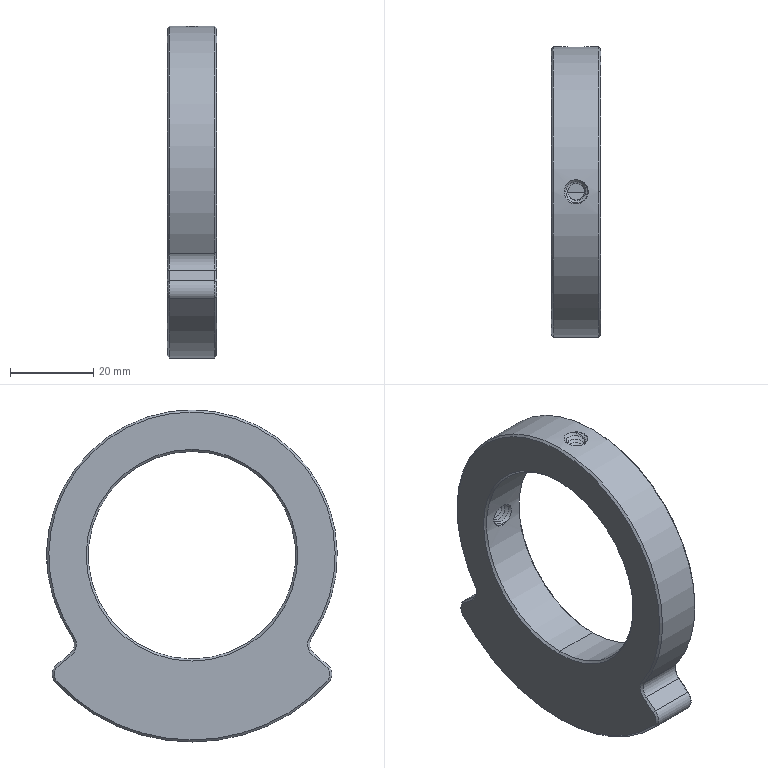Part | SolidWorks | features BaseBody 1 | 1 solid | 89 faces | box 12 x 70 x 80 mm | volume 30669 mm3 | cylinder 43 | spline 20 | cone 18 | plane 8 | commonest cylinder face diameters 4 x34 6 x4 50 x2 90 x2 70 x1